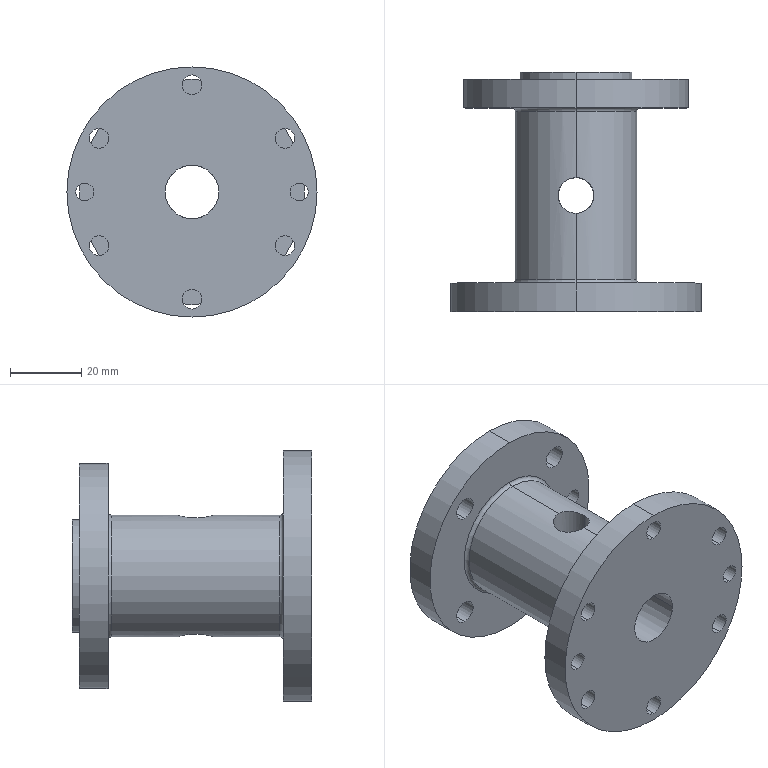Part | SolidWorks | features ICE 5, HoleWzd 2, Cut 1, Extrusion 1, Fillet 1, Helix 1, RevCut 1 | 1 solid | 49 faces | box 70 x 67 x 70 mm | volume 85773 mm3 | cylinder 40 | plane 5 | torus 4 | commonest cylinder face diameters 5.5 x12 6.5 x8 5 x6 10 x4 15 x2 31.5 x2